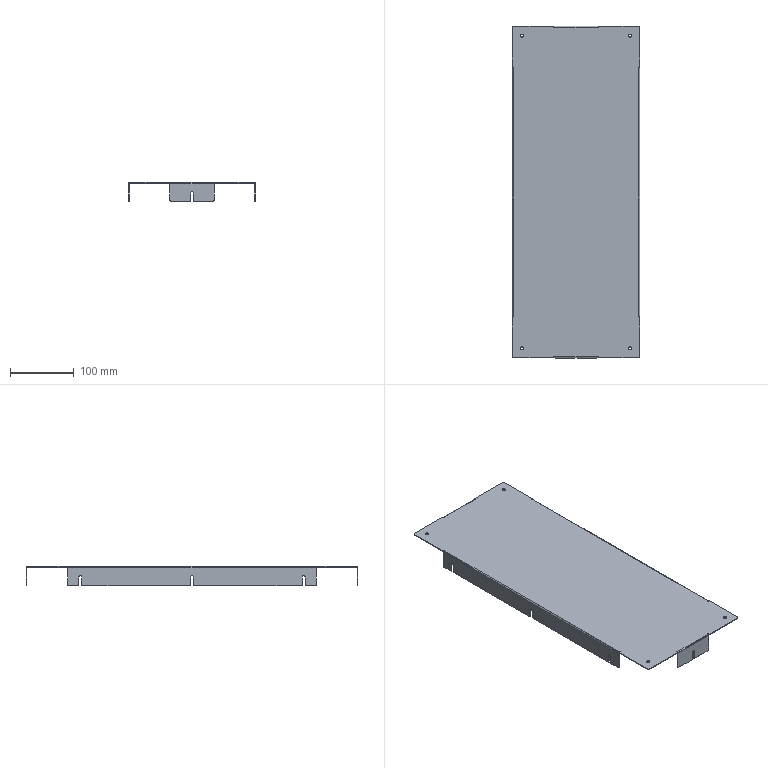Part | STEP file | 1 solid | 128 faces | box 199 x 519 x 30 mm | volume 154248 mm3 | plane 86 | cylinder 42 | commonest cylinder face diameters 4.5 x14 4 x12 5 x8 1.2 x4 3.6 x4